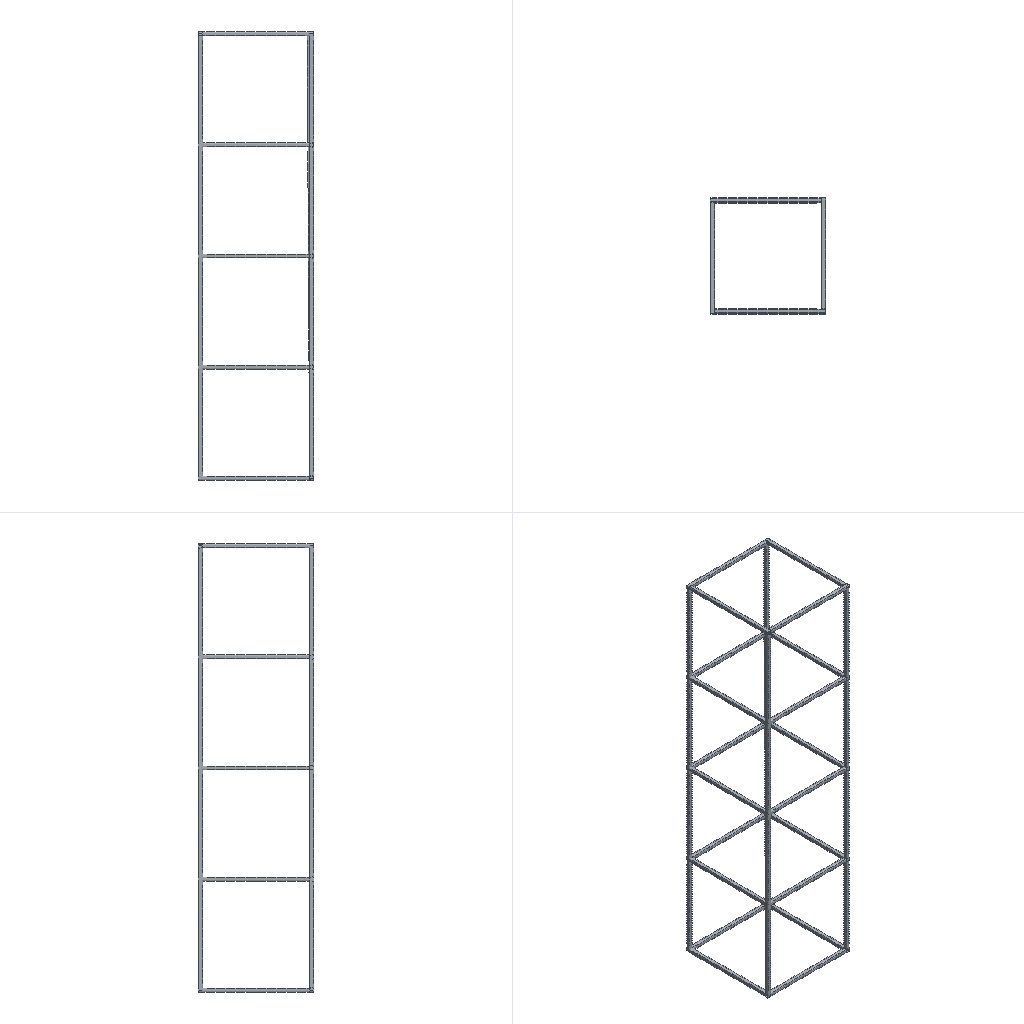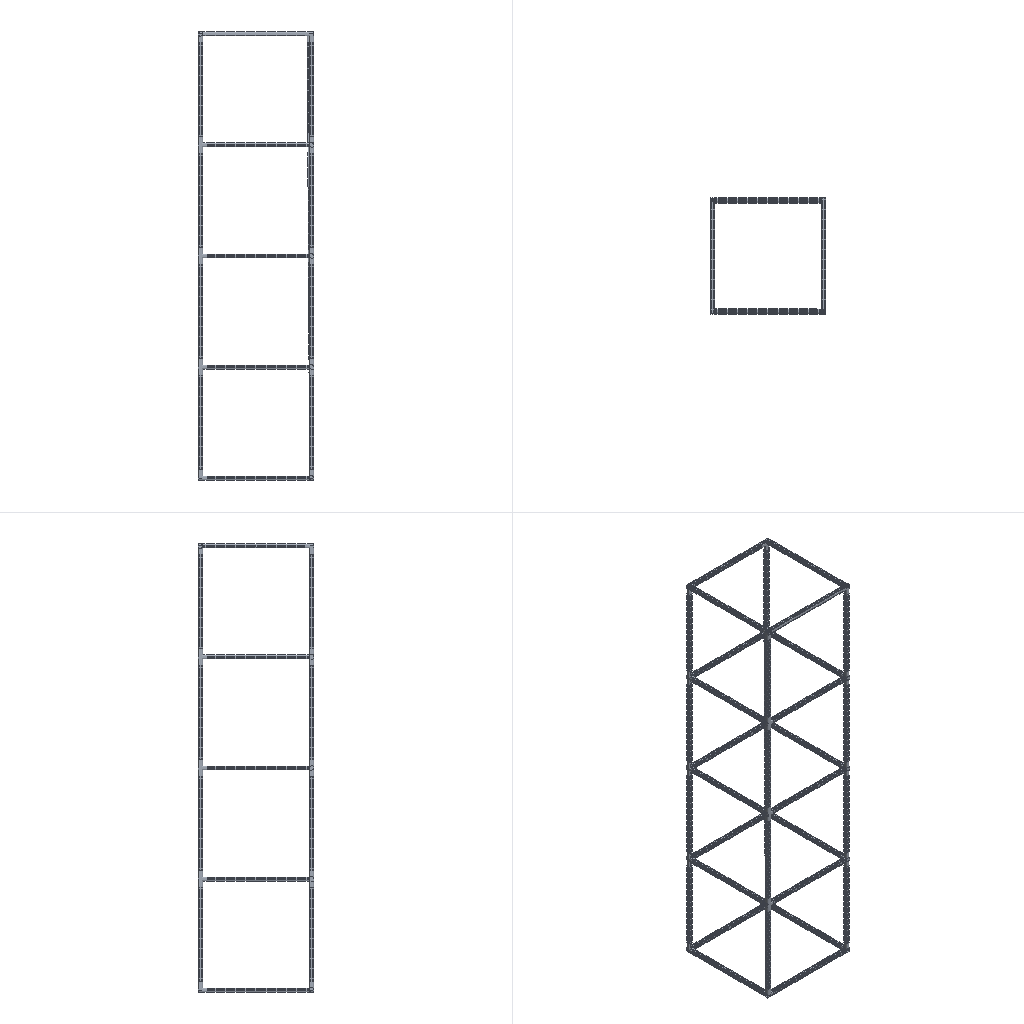Simulation study | ansys workbench
Set-up summary:
category,name,step,type,value,unit,region
solver,ansys_workbench
units,mm-N-s-tonne (MPa),,stated,"/units,MPA"
analysis,deck-1/LS1,,static
load_step,deck-1/LS1,deck-1/LS1,static,nsubst=1; time=1
analysis,deck-2/LS1,,modal,method=lanb; n_modes=6
load_step,deck-2/LS1,deck-2/LS1,modal
mesh,deck-1.dat,,nodes,305448
mesh,deck-1.dat,,elements,62350
element_type,SOLID186,,,43224,,deck-1.dat
element_type,TARGE170,,,8261,,deck-1.dat
element_type,CONTA174,,,8261,,deck-1.dat
element_type,SURF154,,,2604,,deck-1.dat
mesh,deck-2.dat,,nodes,132600
mesh,deck-2.dat,,elements,31364
element_type,SOLID186,,,21674,,deck-2.dat
element_type,TARGE170,,,4845,,deck-2.dat
element_type,CONTA174,,,4845,,deck-2.dat
material,Structural Steel,,E,200000,tonne s^-2 mm^-1
material,Structural Steel,,nu,0.3
material,Structural Steel,,density,7.85e-09,tonne mm^-3
material,Structural Steel,,conductivity,60.5,tonne mm s^-3 C^-1
material,Structural Steel,,specific_heat,4.34e+08,mm^2 s^-2 C^-1
material,Structural Steel,,cte,1.2e-05,C^-1
material,Structural Steel,,permeability,10000
material,Structural Steel,,resistivity,0.00017,ohm mm
material,Structural Steel,,E,200000,tonne s^-2 mm^-1
material,Structural Steel,,nu,0.3
material,Structural Steel,,density,7.85e-09,tonne mm^-3
material,Structural Steel,,conductivity,60.5,tonne mm s^-3 C^-1
material,Structural Steel,,specific_heat,4.34e+08,mm^2 s^-2 C^-1
material,Structural Steel,,cte,1.2e-05,C^-1
material,Structural Steel,,permeability,10000
material,Structural Steel,,resistivity,0.00017,ohm mm
load,Define Force Using Surface Effect Elements,deck-1/LS1,surface-effect pres face 2,-0.0641,,SURF154 #145
bc,Fixed Supports,deck-1/model,fixed,[dofs=ALL],,_FIXEDSU
contact,Contact Region,,bonded (always),element=CONTA174
contact,Contact Region 2,,bonded (always),element=CONTA174
contact,Contact Region 3,,bonded (always),element=CONTA174
contact,Contact Region 4,,bonded (always),element=CONTA174
contact,Contact Region 5,,bonded (always),element=CONTA174
contact,Contact Region 6,,bonded (always),element=CONTA174
contact,Contact Region 7,,bonded (always),element=CONTA174
contact,Contact Region 8,,bonded (always),element=CONTA174
contact,Contact Region 9,,bonded (always),element=CONTA174
contact,Contact Region 10,,bonded (always),element=CONTA174
contact,Contact Region 11,,bonded (always),element=CONTA174
contact,Contact Region 12,,bonded (always),element=CONTA174
contact,Contact Region 13,,bonded (always),element=CONTA174
contact,Contact Region 14,,bonded (always),element=CONTA174
contact,Contact Region 15,,bonded (always),element=CONTA174
contact,Contact Region 16,,bonded (always),element=CONTA174
contact,Contact Region 17,,bonded (always),element=CONTA174
contact,Contact Region 18,,bonded (always),element=CONTA174
contact,Contact Region 19,,bonded (always),element=CONTA174
contact,Contact Region 20,,bonded (always),element=CONTA174
contact,Contact Region 21,,bonded (always),element=CONTA174
contact,Contact Region 22,,bonded (always),element=CONTA174
contact,Contact Region 23,,bonded (always),element=CONTA174
contact,Contact Region 24,,bonded (always),element=CONTA174
contact,Contact Region 25,,bonded (always),element=CONTA174
contact,Contact Region 26,,bonded (always),element=CONTA174
contact,Contact Region 27,,bonded (always),element=CONTA174
contact,Contact Region 28,,bonded (always),element=CONTA174
contact,Contact Region 29,,bonded (always),element=CONTA174
contact,Contact Region 30,,bonded (always),element=CONTA174
contact,Contact Region 31,,bonded (always),element=CONTA174
contact,Contact Region 32,,bonded (always),element=CONTA174
contact,Contact Region 33,,bonded (always),element=CONTA174
contact,Contact Region 34,,bonded (always),element=CONTA174
contact,Contact Region 35,,bonded (always),element=CONTA174
contact,Contact Region 36,,bonded (always),element=CONTA174
contact,Contact Region 37,,bonded (always),element=CONTA174
contact,Contact Region 38,,bonded (always),element=CONTA174
contact,Contact Region 39,,bonded (always),element=CONTA174
contact,Contact Region 40,,bonded (always),element=CONTA174
contact,Contact Region 41,,bonded (always),element=CONTA174
contact,Contact Region 42,,bonded (always),element=CONTA174
contact,Contact Region 43,,bonded (always),element=CONTA174
contact,Contact Region 44,,bonded (always),element=CONTA174
contact,Contact Region 45,,bonded (always),element=CONTA174
contact,Contact Region 46,,bonded (always),element=CONTA174
contact,Contact Region 47,,bonded (always),element=CONTA174
contact,Contact Region 48,,bonded (always),element=CONTA174
contact,Contact Region 49,,bonded (always),element=CONTA174
contact,Contact Region 50,,bonded (always),element=CONTA174
contact,Contact Region 51,,bonded (always),element=CONTA174
contact,Contact Region 52,,bonded (always),element=CONTA174
contact,Contact Region 53,,bonded (always),element=CONTA174
contact,Contact Region 54,,bonded (always),element=CONTA174
contact,Contact Region 55,,bonded (always),element=CONTA174
contact,Contact Region 56,,bonded (always),element=CONTA174
contact,Contact Region 57,,bonded (always),element=CONTA174
contact,Contact Region 58,,bonded (always),element=CONTA174
contact,Contact Region 59,,bonded (always),element=CONTA174
contact,Contact Region 60,,bonded (always),element=CONTA174
contact,Contact Region,,bonded (always),element=CONTA174
contact,Contact Region 2,,bonded (always),element=CONTA174
contact,Contact Region 3,,bonded (always),element=CONTA174
contact,Contact Region 4,,bonded (always),element=CONTA174
contact,Contact Region 5,,bonded (always),element=CONTA174
contact,Contact Region 6,,bonded (always),element=CONTA174
contact,Contact Region 7,,bonded (always),element=CONTA174
contact,Contact Region 8,,bonded (always),element=CONTA174
contact,Contact Region 9,,bonded (always),element=CONTA174
contact,Contact Region 10,,bonded (always),element=CONTA174
contact,Contact Region 11,,bonded (always),element=CONTA174
contact,Contact Region 12,,bonded (always),element=CONTA174
contact,Contact Region 13,,bonded (always),element=CONTA174
contact,Contact Region 14,,bonded (always),element=CONTA174
contact,Contact Region 15,,bonded (always),element=CONTA174
contact,Contact Region 16,,bonded (always),element=CONTA174
contact,Contact Region 17,,bonded (always),element=CONTA174
contact,Contact Region 18,,bonded (always),element=CONTA174
contact,Contact Region 19,,bonded (always),element=CONTA174
contact,Contact Region 20,,bonded (always),element=CONTA174
contact,Contact Region 21,,bonded (always),element=CONTA174
contact,Contact Region 22,,bonded (always),element=CONTA174
contact,Contact Region 23,,bonded (always),element=CONTA174
contact,Contact Region 24,,bonded (always),element=CONTA174
contact,Contact Region 25,,bonded (always),element=CONTA174
contact,Contact Region 26,,bonded (always),element=CONTA174
contact,Contact Region 27,,bonded (always),element=CONTA174
contact,Contact Region 28,,bonded (always),element=CONTA174
contact,Contact Region 29,,bonded (always),element=CONTA174
contact,Contact Region 30,,bonded (always),element=CONTA174
contact,Contact Region 31,,bonded (always),element=CONTA174
contact,Contact Region 32,,bonded (always),element=CONTA174
contact,Contact Region 33,,bonded (always),element=CONTA174
contact,Contact Region 34,,bonded (always),element=CONTA174
contact,Contact Region 35,,bonded (always),element=CONTA174
contact,Contact Region 36,,bonded (always),element=CONTA174
contact,Contact Region 37,,bonded (always),element=CONTA174
contact,Contact Region 38,,bonded (always),element=CONTA174
contact,Contact Region 39,,bonded (always),element=CONTA174
contact,Contact Region 40,,bonded (always),element=CONTA174
contact,Contact Region 41,,bonded (always),element=CONTA174
contact,Contact Region 42,,bonded (always),element=CONTA174
contact,Contact Region 43,,bonded (always),element=CONTA174
contact,Contact Region 44,,bonded (always),element=CONTA174
contact,Contact Region 45,,bonded (always),element=CONTA174
contact,Contact Region 46,,bonded (always),element=CONTA174
contact,Contact Region 47,,bonded (always),element=CONTA174
contact,Contact Region 48,,bonded (always),element=CONTA174
contact,Contact Region 49,,bonded (always),element=CONTA174
contact,Contact Region 50,,bonded (always),element=CONTA174
contact,Contact Region 51,,bonded (always),element=CONTA174
contact,Contact Region 52,,bonded (always),element=CONTA174
contact,Contact Region 53,,bonded (always),element=CONTA174
contact,Contact Region 54,,bonded (always),element=CONTA174
contact,Contact Region 55,,bonded (always),element=CONTA174
contact,Contact Region 56,,bonded (always),element=CONTA174
contact,Contact Region 57,,bonded (always),element=CONTA174
contact,Contact Region 58,,bonded (always),element=CONTA174
contact,Contact Region 59,,bonded (always),element=CONTA174
contact,Contact Region 60,,bonded (always),element=CONTA174
named_set,_FIXEDSU,,node,2836
Results summary:
result,analyses[0].index,,,1
result,analyses[0].system,,,SYS
result,analyses[0].deck,,,deck-1.dat
result,analyses[0].solve_status,,,completed
result,analyses[0].analysis_type,,,static
result,analyses[0].physics,,,mechanical
result,analyses[0].unit_system,,,"NMM: mm, ton, N, s, mV, mA, degC"
result,analyses[0].n_sets,,,1
result,analyses[0].load_steps[0].set,set=1,,1
result,analyses[0].load_steps[0].time_or_freq,set=1,,1
result,analyses[0].load_steps[0].max_displacement_magnitude,set=1,,42.867
result,analyses[0].load_steps[0].max_von_mises_nodal,set=1,,2464.27
result,analyses[0].load_steps[0].reaction_force_sum_xyz[1],set=1,,-0.0006178
result,analyses[0].load_steps[0].reaction_force_sum_xyz[2],set=1,,5000
result,analyses[0].load_steps[0].reaction_force_sum_xyz[3],set=1,,-0.0008188
result,analyses[1].index,,,2
result,analyses[1].system,,,SYS-1
result,analyses[1].deck,,,deck-2.dat
result,analyses[1].solve_status,,,completed
result,analyses[1].analysis_type,,,modal
result,analyses[1].physics,,,mechanical
result,analyses[1].unit_system,,,"NMM: mm, ton, N, s, mV, mA, degC"
result,analyses[1].n_sets,,,6
result,analyses[1].modal_frequencies_hz[1],,,0
result,analyses[1].modal_frequencies_hz[2],,,0
result,analyses[1].modal_frequencies_hz[3],,,0.007522
result,analyses[1].modal_frequencies_hz[4],,,27.706
result,analyses[1].modal_frequencies_hz[5],,,27.856
result,analyses[1].modal_frequencies_hz[6],,,60.344